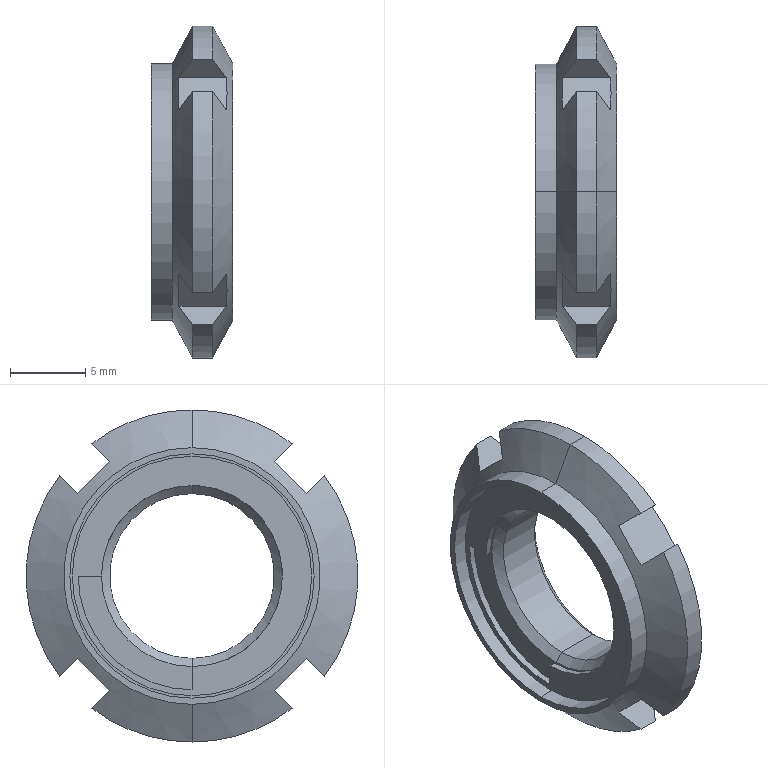Part | STEP file | Lock nut FUNT12_MISUMI | 2 solids | 42 faces | box 5.4 x 22 x 22 mm | volume 932.86 mm3 | plane 19 | cylinder 15 | cone 8 | commonest cylinder face diameters 22 x5 10.917 x2 15.867 x2 16.19 x2 17 x2 12 x1
STEP:
#1=CARTESIAN_POINT('',(-4.14,0.,-7.933));
#2=VERTEX_POINT('',#1);
#3=CARTESIAN_POINT('',(-4.14,0.,7.933));
#4=VERTEX_POINT('',#3);
#5=CARTESIAN_POINT('',(-4.14,0.,0.));
#6=DIRECTION('',(1.,0.,0.));
#7=DIRECTION('',(0.,0.,1.));
#8=AXIS2_PLACEMENT_3D('',#5,#6,#7);
#9=CIRCLE('',#8,7.933);
#10=EDGE_CURVE('',#2,#4,#9,.T.);
#11=ORIENTED_EDGE('',*,*,#10,.F.);
#12=CARTESIAN_POINT('',(-4.56,0.,-7.933));
#13=VERTEX_POINT('',#12);
#14=CARTESIAN_POINT('',(-4.14,0.,-7.933));
#15=DIRECTION('',(-1.,0.,0.));
#16=VECTOR('',#15,1000.);
#17=LINE('',#14,#16);
#18=EDGE_CURVE('',#2,#13,#17,.T.);
#19=ORIENTED_EDGE('',*,*,#18,.T.);
#20=CARTESIAN_POINT('',(-4.56,0.,7.933));
#21=VERTEX_POINT('',#20);
#22=CARTESIAN_POINT('',(-4.56,0.,0.));
#23=DIRECTION('',(1.,0.,0.));
#24=DIRECTION('',(0.,0.,1.));
#25=AXIS2_PLACEMENT_3D('',#22,#23,#24);
#26=CIRCLE('',#25,7.933);
#27=EDGE_CURVE('',#13,#21,#26,.T.);
#28=ORIENTED_EDGE('',*,*,#27,.T.);
#29=CARTESIAN_POINT('',(-4.14,0.,7.933));
#30=DIRECTION('',(-1.,0.,0.));
#31=VECTOR('',#30,1000.);
#32=LINE('',#29,#31);
#33=EDGE_CURVE('',#4,#21,#32,.T.);
#34=ORIENTED_EDGE('',*,*,#33,.F.);
#35=EDGE_LOOP('',(#11,#19,#28,#34));
#36=FACE_OUTER_BOUND('',#35,.T.);
#37=CARTESIAN_POINT('',(-4.14,0.,0.));
#38=DIRECTION('',(-1.,0.,0.));
#39=DIRECTION('',(0.,0.,1.));
#40=AXIS2_PLACEMENT_3D('',#37,#38,#39);
#41=CYLINDRICAL_SURFACE('',#40,7.933);
#42=ADVANCED_FACE('',(#36),#41,.T.);
#43=CARTESIAN_POINT('',(-4.14,0.,0.));
#44=DIRECTION('',(1.,0.,0.));
#45=DIRECTION('',(0.,0.,1.));
#46=AXIS2_PLACEMENT_3D('',#43,#44,#45);
#47=CIRCLE('',#46,7.933);
#48=EDGE_CURVE('',#4,#2,#47,.T.);
#49=ORIENTED_EDGE('',*,*,#48,.T.);
#50=ORIENTED_EDGE('',*,*,#10,.T.);
#51=EDGE_LOOP('',(#49,#50));
#52=FACE_OUTER_BOUND('',#51,.T.);
#53=CARTESIAN_POINT('',(-4.14,0.,-7.537));
#54=VERTEX_POINT('',#53);
#55=CARTESIAN_POINT('',(-4.14,0.,-6.));
#56=VERTEX_POINT('',#55);
#57=CARTESIAN_POINT('',(-4.14,0.,7.933));
#58=DIRECTION('',(0.,0.,1.));
#59=VECTOR('',#58,1000.);
#60=LINE('',#57,#59);
#61=EDGE_CURVE('',#54,#56,#60,.T.);
#62=ORIENTED_EDGE('',*,*,#61,.T.);
#63=CARTESIAN_POINT('',(-4.14,6.,0.));
#64=VERTEX_POINT('',#63);
#65=CARTESIAN_POINT('',(-4.14,0.,0.));
#66=DIRECTION('',(-1.,0.,0.));
#67=DIRECTION('',(0.,0.,-1.));
#68=AXIS2_PLACEMENT_3D('',#65,#66,#67);
#69=CIRCLE('',#68,6.);
#70=EDGE_CURVE('',#56,#64,#69,.T.);
#71=ORIENTED_EDGE('',*,*,#70,.T.);
#72=CARTESIAN_POINT('',(-4.14,7.537,0.));
#73=VERTEX_POINT('',#72);
#74=CARTESIAN_POINT('',(-4.14,-7.933,0.));
#75=DIRECTION('',(0.,1.,0.));
#76=VECTOR('',#75,1000.);
#77=LINE('',#74,#76);
#78=EDGE_CURVE('',#64,#73,#77,.T.);
#79=ORIENTED_EDGE('',*,*,#78,.T.);
#80=CARTESIAN_POINT('',(-4.14,0.,0.));
#81=DIRECTION('',(-1.,0.,0.));
#82=DIRECTION('',(0.,0.,-1.));
#83=AXIS2_PLACEMENT_3D('',#80,#81,#82);
#84=CIRCLE('',#83,7.537);
#85=EDGE_CURVE('',#73,#54,#84,.T.);
#86=ORIENTED_EDGE('',*,*,#85,.T.);
#87=EDGE_LOOP('',(#62,#71,#79,#86));
#88=FACE_BOUND('',#87,.T.);
#89=CARTESIAN_POINT('',(-4.14,-7.933,7.933));
#90=DIRECTION('',(1.,0.,0.));
#91=DIRECTION('',(0.,0.,-1.));
#92=AXIS2_PLACEMENT_3D('',#89,#90,#91);
#93=PLANE('',#92);
#94=ADVANCED_FACE('',(#52,#88),#93,.T.);
#95=ORIENTED_EDGE('',*,*,#18,.F.);
#96=ORIENTED_EDGE('',*,*,#48,.F.);
#97=ORIENTED_EDGE('',*,*,#33,.T.);
#98=CARTESIAN_POINT('',(-4.56,0.,0.));
#99=DIRECTION('',(1.,0.,0.));
#100=DIRECTION('',(0.,0.,1.));
#101=AXIS2_PLACEMENT_3D('',#98,#99,#100);
#102=CIRCLE('',#101,7.933);
#103=EDGE_CURVE('',#21,#13,#102,.T.);
#104=ORIENTED_EDGE('',*,*,#103,.T.);
#105=EDGE_LOOP('',(#95,#96,#97,#104));
#106=FACE_OUTER_BOUND('',#105,.T.);
#107=CARTESIAN_POINT('',(-4.14,0.,0.));
#108=DIRECTION('',(-1.,0.,0.));
#109=DIRECTION('',(0.,0.,1.));
#110=AXIS2_PLACEMENT_3D('',#107,#108,#109);
#111=CYLINDRICAL_SURFACE('',#110,7.933);
#112=ADVANCED_FACE('',(#106),#111,.T.);
#113=ORIENTED_EDGE('',*,*,#70,.F.);
#114=CARTESIAN_POINT('',(-4.56,0.,-6.));
#115=VERTEX_POINT('',#114);
#116=CARTESIAN_POINT('',(-4.56,0.,-6.));
#117=DIRECTION('',(1.,0.,0.));
#118=VECTOR('',#117,1000.);
#119=LINE('',#116,#118);
#120=EDGE_CURVE('',#115,#56,#119,.T.);
#121=ORIENTED_EDGE('',*,*,#120,.F.);
#122=CARTESIAN_POINT('',(-4.56,6.,0.));
#123=VERTEX_POINT('',#122);
#124=CARTESIAN_POINT('',(-4.56,0.,0.));
#125=DIRECTION('',(1.,0.,0.));
#126=DIRECTION('',(0.,0.,-1.));
#127=AXIS2_PLACEMENT_3D('',#124,#125,#126);
#128=CIRCLE('',#127,6.);
#129=EDGE_CURVE('',#123,#115,#128,.T.);
#130=ORIENTED_EDGE('',*,*,#129,.F.);
#131=CARTESIAN_POINT('',(-4.56,6.,0.));
#132=DIRECTION('',(-1.,0.,0.));
#133=VECTOR('',#132,1000.);
#134=LINE('',#131,#133);
#135=EDGE_CURVE('',#64,#123,#134,.T.);
#136=ORIENTED_EDGE('',*,*,#135,.F.);
#137=EDGE_LOOP('',(#113,#121,#130,#136));
#138=FACE_OUTER_BOUND('',#137,.T.);
#139=CARTESIAN_POINT('',(-4.56,0.,0.));
#140=DIRECTION('',(1.,0.,0.));
#141=DIRECTION('',(0.,0.,-1.));
#142=AXIS2_PLACEMENT_3D('',#139,#140,#141);
#143=CYLINDRICAL_SURFACE('',#142,6.);
#144=ADVANCED_FACE('',(#138),#143,.F.);
#145=ORIENTED_EDGE('',*,*,#120,.T.);
#146=ORIENTED_EDGE('',*,*,#61,.F.);
#147=CARTESIAN_POINT('',(-4.56,0.,-7.537));
#148=VERTEX_POINT('',#147);
#149=CARTESIAN_POINT('',(-4.14,0.,-7.537));
#150=DIRECTION('',(-1.,0.,0.));
#151=VECTOR('',#150,1000.);
#152=LINE('',#149,#151);
#153=EDGE_CURVE('',#54,#148,#152,.T.);
#154=ORIENTED_EDGE('',*,*,#153,.T.);
#155=CARTESIAN_POINT('',(-4.56,0.,-7.537));
#156=DIRECTION('',(0.,0.,1.));
#157=VECTOR('',#156,1000.);
#158=LINE('',#155,#157);
#159=EDGE_CURVE('',#148,#115,#158,.T.);
#160=ORIENTED_EDGE('',*,*,#159,.T.);
#161=EDGE_LOOP('',(#145,#146,#154,#160));
#162=FACE_OUTER_BOUND('',#161,.T.);
#163=CARTESIAN_POINT('',(-4.14,0.,-7.537));
#164=DIRECTION('',(0.,1.,0.));
#165=DIRECTION('',(0.,0.,1.));
#166=AXIS2_PLACEMENT_3D('',#163,#164,#165);
#167=PLANE('',#166);
#168=ADVANCED_FACE('',(#162),#167,.T.);
#169=CARTESIAN_POINT('',(-4.56,7.537,0.));
#170=VERTEX_POINT('',#169);
#171=CARTESIAN_POINT('',(-4.56,7.537,0.));
#172=DIRECTION('',(1.,0.,0.));
#173=VECTOR('',#172,1000.);
#174=LINE('',#171,#173);
#175=EDGE_CURVE('',#170,#73,#174,.T.);
#176=ORIENTED_EDGE('',*,*,#175,.F.);
#177=CARTESIAN_POINT('',(-4.56,0.,0.));
#178=DIRECTION('',(1.,0.,0.));
#179=DIRECTION('',(0.,0.,-1.));
#180=AXIS2_PLACEMENT_3D('',#177,#178,#179);
#181=CIRCLE('',#180,7.537);
#182=EDGE_CURVE('',#148,#170,#181,.T.);
#183=ORIENTED_EDGE('',*,*,#182,.F.);
#184=ORIENTED_EDGE('',*,*,#153,.F.);
#185=ORIENTED_EDGE('',*,*,#85,.F.);
#186=EDGE_LOOP('',(#176,#183,#184,#185));
#187=FACE_OUTER_BOUND('',#186,.T.);
#188=CARTESIAN_POINT('',(-4.56,0.,0.));
#189=DIRECTION('',(1.,0.,0.));
#190=DIRECTION('',(0.,0.,-1.));
#191=AXIS2_PLACEMENT_3D('',#188,#189,#190);
#192=CYLINDRICAL_SURFACE('',#191,7.537);
#193=ADVANCED_FACE('',(#187),#192,.F.);
#194=ORIENTED_EDGE('',*,*,#175,.T.);
#195=ORIENTED_EDGE('',*,*,#78,.F.);
#196=ORIENTED_EDGE('',*,*,#135,.T.);
#197=CARTESIAN_POINT('',(-4.56,6.,0.));
#198=DIRECTION('',(0.,1.,0.));
#199=VECTOR('',#198,1000.);
#200=LINE('',#197,#199);
#201=EDGE_CURVE('',#123,#170,#200,.T.);
#202=ORIENTED_EDGE('',*,*,#201,.T.);
#203=EDGE_LOOP('',(#194,#195,#196,#202));
#204=FACE_OUTER_BOUND('',#203,.T.);
#205=CARTESIAN_POINT('',(-4.14,6.,0.));
#206=DIRECTION('',(0.,0.,-1.));
#207=DIRECTION('',(0.,1.,0.));
#208=AXIS2_PLACEMENT_3D('',#205,#206,#207);
#209=PLANE('',#208);
#210=ADVANCED_FACE('',(#204),#209,.T.);
#211=ORIENTED_EDGE('',*,*,#103,.F.);
#212=ORIENTED_EDGE('',*,*,#27,.F.);
#213=EDGE_LOOP('',(#211,#212));
#214=FACE_OUTER_BOUND('',#213,.T.);
#215=ORIENTED_EDGE('',*,*,#159,.F.);
#216=ORIENTED_EDGE('',*,*,#182,.T.);
#217=ORIENTED_EDGE('',*,*,#201,.F.);
#218=ORIENTED_EDGE('',*,*,#129,.T.);
#219=EDGE_LOOP('',(#215,#216,#217,#218));
#220=FACE_BOUND('',#219,.T.);
#221=CARTESIAN_POINT('',(-4.56,-7.933,-7.933));
#222=DIRECTION('',(-1.,0.,0.));
#223=DIRECTION('',(0.,0.,1.));
#224=AXIS2_PLACEMENT_3D('',#221,#222,#223);
#225=PLANE('',#224);
#226=ADVANCED_FACE('',(#214,#220),#225,.T.);
#227=CLOSED_SHELL('',(#42,#94,#112,#144,#168,#193,#210,#226));
#228=MANIFOLD_SOLID_BREP('',#227);
#229=CARTESIAN_POINT('',(0.,0.,-8.5));
#230=VERTEX_POINT('',#229);
#231=CARTESIAN_POINT('',(0.,0.,8.5));
#232=VERTEX_POINT('',#231);
#233=CARTESIAN_POINT('',(0.,0.,0.));
#234=DIRECTION('',(1.,0.,0.));
#235=DIRECTION('',(0.,0.,1.));
#236=AXIS2_PLACEMENT_3D('',#233,#234,#235);
#237=CIRCLE('',#236,8.5);
#238=EDGE_CURVE('',#230,#232,#237,.T.);
#239=ORIENTED_EDGE('',*,*,#238,.F.);
#240=CARTESIAN_POINT('',(-1.333,0.,-11.));
#241=VERTEX_POINT('',#240);
#242=CARTESIAN_POINT('',(-1.333,0.,-11.));
#243=DIRECTION('',(-0.4706,0.,-0.8824));
#244=VECTOR('',#243,1000.);
#245=LINE('',#242,#244);
#246=EDGE_CURVE('',#230,#241,#245,.T.);
#247=ORIENTED_EDGE('',*,*,#246,.T.);
#248=CARTESIAN_POINT('',(-1.333,6.645,-8.766));
#249=VERTEX_POINT('',#248);
#250=CARTESIAN_POINT('',(-1.333,0.,0.));
#251=DIRECTION('',(1.,0.,0.));
#252=DIRECTION('',(0.,0.,1.));
#253=AXIS2_PLACEMENT_3D('',#250,#251,#252);
#254=CIRCLE('',#253,11.);
#255=EDGE_CURVE('',#241,#249,#254,.T.);
#256=ORIENTED_EDGE('',*,*,#255,.T.);
#257=CARTESIAN_POINT('',(-0.4381,5.445,-7.566));
#258=VERTEX_POINT('',#257);
#259=CARTESIAN_POINT('',(-1.333,6.645,-8.766));
#260=CARTESIAN_POINT('',(-1.035,6.245,-8.366));
#261=CARTESIAN_POINT('',(-0.7361,5.845,-7.966));
#262=CARTESIAN_POINT('',(-0.4381,5.445,-7.566));
#263=B_SPLINE_CURVE_WITH_KNOTS('',3,(#259,#260,#261,#262),.UNSPECIFIED.,.F.,.F.,(4,4),(0.,0.001919),.UNSPECIFIED.);
#264=EDGE_CURVE('',#249,#258,#263,.T.);
#265=ORIENTED_EDGE('',*,*,#264,.T.);
#266=CARTESIAN_POINT('',(-0.4381,7.566,-5.445));
#267=VERTEX_POINT('',#266);
#268=CARTESIAN_POINT('',(-0.4381,5.445,-7.566));
#269=CARTESIAN_POINT('',(-0.3523,6.152,-6.859));
#270=CARTESIAN_POINT('',(-0.3523,6.859,-6.152));
#271=CARTESIAN_POINT('',(-0.4381,7.566,-5.445));
#272=B_SPLINE_CURVE_WITH_KNOTS('',3,(#268,#269,#270,#271),.UNSPECIFIED.,.F.,.F.,(4,4),(0.,0.003),.UNSPECIFIED.);
#273=EDGE_CURVE('',#258,#267,#272,.T.);
#274=ORIENTED_EDGE('',*,*,#273,.T.);
#275=CARTESIAN_POINT('',(-1.333,8.766,-6.645));
#276=VERTEX_POINT('',#275);
#277=CARTESIAN_POINT('',(-0.4381,7.566,-5.445));
#278=CARTESIAN_POINT('',(-0.7361,7.966,-5.845));
#279=CARTESIAN_POINT('',(-1.035,8.366,-6.245));
#280=CARTESIAN_POINT('',(-1.333,8.766,-6.645));
#281=B_SPLINE_CURVE_WITH_KNOTS('',3,(#277,#278,#279,#280),.UNSPECIFIED.,.F.,.F.,(4,4),(0.,0.001919),.UNSPECIFIED.);
#282=EDGE_CURVE('',#267,#276,#281,.T.);
#283=ORIENTED_EDGE('',*,*,#282,.T.);
#284=CARTESIAN_POINT('',(-1.333,8.766,6.645));
#285=VERTEX_POINT('',#284);
#286=CARTESIAN_POINT('',(-1.333,0.,0.));
#287=DIRECTION('',(1.,0.,0.));
#288=DIRECTION('',(0.,0.,1.));
#289=AXIS2_PLACEMENT_3D('',#286,#287,#288);
#290=CIRCLE('',#289,11.);
#291=EDGE_CURVE('',#276,#285,#290,.T.);
#292=ORIENTED_EDGE('',*,*,#291,.T.);
#293=CARTESIAN_POINT('',(-0.4381,7.566,5.445));
#294=VERTEX_POINT('',#293);
#295=CARTESIAN_POINT('',(-1.333,8.766,6.645));
#296=CARTESIAN_POINT('',(-1.035,8.366,6.245));
#297=CARTESIAN_POINT('',(-0.7361,7.966,5.845));
#298=CARTESIAN_POINT('',(-0.4381,7.566,5.445));
#299=B_SPLINE_CURVE_WITH_KNOTS('',3,(#295,#296,#297,#298),.UNSPECIFIED.,.F.,.F.,(4,4),(0.,0.001919),.UNSPECIFIED.);
#300=EDGE_CURVE('',#285,#294,#299,.T.);
#301=ORIENTED_EDGE('',*,*,#300,.T.);
#302=CARTESIAN_POINT('',(-0.4381,5.445,7.566));
#303=VERTEX_POINT('',#302);
#304=CARTESIAN_POINT('',(-0.4381,7.566,5.445));
#305=CARTESIAN_POINT('',(-0.3523,6.859,6.152));
#306=CARTESIAN_POINT('',(-0.3523,6.152,6.859));
#307=CARTESIAN_POINT('',(-0.4381,5.445,7.566));
#308=B_SPLINE_CURVE_WITH_KNOTS('',3,(#304,#305,#306,#307),.UNSPECIFIED.,.F.,.F.,(4,4),(0.,0.003),.UNSPECIFIED.);
#309=EDGE_CURVE('',#294,#303,#308,.T.);
#310=ORIENTED_EDGE('',*,*,#309,.T.);
#311=CARTESIAN_POINT('',(-1.333,6.645,8.766));
#312=VERTEX_POINT('',#311);
#313=CARTESIAN_POINT('',(-0.4381,5.445,7.566));
#314=CARTESIAN_POINT('',(-0.7361,5.845,7.966));
#315=CARTESIAN_POINT('',(-1.035,6.245,8.366));
#316=CARTESIAN_POINT('',(-1.333,6.645,8.766));
#317=B_SPLINE_CURVE_WITH_KNOTS('',3,(#313,#314,#315,#316),.UNSPECIFIED.,.F.,.F.,(4,4),(0.,0.001919),.UNSPECIFIED.);
#318=EDGE_CURVE('',#303,#312,#317,.T.);
#319=ORIENTED_EDGE('',*,*,#318,.T.);
#320=CARTESIAN_POINT('',(-1.333,0.,11.));
#321=VERTEX_POINT('',#320);
#322=CARTESIAN_POINT('',(-1.333,0.,0.));
#323=DIRECTION('',(1.,0.,0.));
#324=DIRECTION('',(0.,0.,1.));
#325=AXIS2_PLACEMENT_3D('',#322,#323,#324);
#326=CIRCLE('',#325,11.);
#327=EDGE_CURVE('',#312,#321,#326,.T.);
#328=ORIENTED_EDGE('',*,*,#327,.T.);
#329=CARTESIAN_POINT('',(-1.333,0.,11.));
#330=DIRECTION('',(-0.4706,0.,0.8824));
#331=VECTOR('',#330,1000.);
#332=LINE('',#329,#331);
#333=EDGE_CURVE('',#232,#321,#332,.T.);
#334=ORIENTED_EDGE('',*,*,#333,.F.);
#335=EDGE_LOOP('',(#239,#247,#256,#265,#274,#283,#292,#301,#310,#319,#328,#334));
#336=FACE_OUTER_BOUND('',#335,.T.);
#337=CARTESIAN_POINT('',(-1.333,0.,0.));
#338=DIRECTION('',(-1.,0.,0.));
#339=DIRECTION('',(0.,0.,1.));
#340=AXIS2_PLACEMENT_3D('',#337,#338,#339);
#341=CONICAL_SURFACE('',#340,11.,1.081);
#342=ADVANCED_FACE('',(#336),#341,.T.);
#343=CARTESIAN_POINT('',(-0.5415,0.,5.459));
#344=VERTEX_POINT('',#343);
#345=CARTESIAN_POINT('',(-0.5415,0.,-5.459));
#346=VERTEX_POINT('',#345);
#347=CARTESIAN_POINT('',(-0.5415,0.,0.));
#348=DIRECTION('',(1.,0.,0.));
#349=DIRECTION('',(0.,0.,-1.));
#350=AXIS2_PLACEMENT_3D('',#347,#348,#349);
#351=CIRCLE('',#350,5.459);
#352=EDGE_CURVE('',#344,#346,#351,.T.);
#353=ORIENTED_EDGE('',*,*,#352,.F.);
#354=CARTESIAN_POINT('',(0.,0.,6.));
#355=VERTEX_POINT('',#354);
#356=CARTESIAN_POINT('',(0.,0.,6.));
#357=DIRECTION('',(0.7071,0.,0.7071));
#358=VECTOR('',#357,1000.);
#359=LINE('',#356,#358);
#360=EDGE_CURVE('',#344,#355,#359,.T.);
#361=ORIENTED_EDGE('',*,*,#360,.T.);
#362=CARTESIAN_POINT('',(0.,0.,-6.));
#363=VERTEX_POINT('',#362);
#364=CARTESIAN_POINT('',(0.,0.,0.));
#365=DIRECTION('',(-1.,0.,0.));
#366=DIRECTION('',(0.,0.,-1.));
#367=AXIS2_PLACEMENT_3D('',#364,#365,#366);
#368=CIRCLE('',#367,6.);
#369=EDGE_CURVE('',#363,#355,#368,.T.);
#370=ORIENTED_EDGE('',*,*,#369,.F.);
#371=CARTESIAN_POINT('',(0.,0.,-6.));
#372=DIRECTION('',(0.7071,0.,-0.7071));
#373=VECTOR('',#372,1000.);
#374=LINE('',#371,#373);
#375=EDGE_CURVE('',#346,#363,#374,.T.);
#376=ORIENTED_EDGE('',*,*,#375,.F.);
#377=EDGE_LOOP('',(#353,#361,#370,#376));
#378=FACE_OUTER_BOUND('',#377,.T.);
#379=CARTESIAN_POINT('',(0.,0.,0.));
#380=DIRECTION('',(1.,0.,0.));
#381=DIRECTION('',(0.,0.,-1.));
#382=AXIS2_PLACEMENT_3D('',#379,#380,#381);
#383=CONICAL_SURFACE('',#382,6.,0.7854);
#384=ADVANCED_FACE('',(#378),#383,.F.);
#385=CARTESIAN_POINT('',(-1.333,-6.645,8.766));
#386=VERTEX_POINT('',#385);
#387=CARTESIAN_POINT('',(-1.333,0.,0.));
#388=DIRECTION('',(1.,0.,0.));
#389=DIRECTION('',(0.,0.,1.));
#390=AXIS2_PLACEMENT_3D('',#387,#388,#389);
#391=CIRCLE('',#390,11.);
#392=EDGE_CURVE('',#321,#386,#391,.T.);
#393=ORIENTED_EDGE('',*,*,#392,.F.);
#394=CARTESIAN_POINT('',(-2.667,0.,11.));
#395=VERTEX_POINT('',#394);
#396=CARTESIAN_POINT('',(-1.333,0.,11.));
#397=DIRECTION('',(-1.,0.,0.));
#398=VECTOR('',#397,1000.);
#399=LINE('',#396,#398);
#400=EDGE_CURVE('',#321,#395,#399,.T.);
#401=ORIENTED_EDGE('',*,*,#400,.T.);
#402=CARTESIAN_POINT('',(-2.667,-6.645,8.766));
#403=VERTEX_POINT('',#402);
#404=CARTESIAN_POINT('',(-2.667,0.,0.));
#405=DIRECTION('',(1.,0.,0.));
#406=DIRECTION('',(0.,0.,1.));
#407=AXIS2_PLACEMENT_3D('',#404,#405,#406);
#408=CIRCLE('',#407,11.);
#409=EDGE_CURVE('',#395,#403,#408,.T.);
#410=ORIENTED_EDGE('',*,*,#409,.T.);
#411=CARTESIAN_POINT('',(-3.562,-6.645,8.766));
#412=DIRECTION('',(-1.,0.,0.));
#413=VECTOR('',#412,1000.);
#414=LINE('',#411,#413);
#415=EDGE_CURVE('',#386,#403,#414,.T.);
#416=ORIENTED_EDGE('',*,*,#415,.F.);
#417=EDGE_LOOP('',(#393,#401,#410,#416));
#418=FACE_OUTER_BOUND('',#417,.T.);
#419=CARTESIAN_POINT('',(-1.333,0.,0.));
#420=DIRECTION('',(-1.,0.,0.));
#421=DIRECTION('',(0.,0.,1.));
#422=AXIS2_PLACEMENT_3D('',#419,#420,#421);
#423=CYLINDRICAL_SURFACE('',#422,11.);
#424=ADVANCED_FACE('',(#418),#423,.T.);
#425=ORIENTED_EDGE('',*,*,#352,.T.);
#426=CARTESIAN_POINT('',(-3.459,0.,-5.459));
#427=VERTEX_POINT('',#426);
#428=CARTESIAN_POINT('',(-0.5415,0.,-5.459));
#429=DIRECTION('',(-1.,0.,0.));
#430=VECTOR('',#429,1000.);
#431=LINE('',#428,#430);
#432=EDGE_CURVE('',#346,#427,#431,.T.);
#433=ORIENTED_EDGE('',*,*,#432,.T.);
#434=CARTESIAN_POINT('',(-3.459,0.,5.458));
#435=VERTEX_POINT('',#434);
#436=CARTESIAN_POINT('',(-3.459,0.,0.));
#437=DIRECTION('',(1.,0.,0.));
#438=DIRECTION('',(0.,0.,1.));
#439=AXIS2_PLACEMENT_3D('',#436,#437,#438);
#440=CIRCLE('',#439,5.458);
#441=EDGE_CURVE('',#435,#427,#440,.T.);
#442=ORIENTED_EDGE('',*,*,#441,.F.);
#443=CARTESIAN_POINT('',(-0.5415,0.,5.458));
#444=DIRECTION('',(-1.,0.,0.));
#445=VECTOR('',#444,1000.);
#446=LINE('',#443,#445);
#447=EDGE_CURVE('',#344,#435,#446,.T.);
#448=ORIENTED_EDGE('',*,*,#447,.F.);
#449=EDGE_LOOP('',(#425,#433,#442,#448));
#450=FACE_OUTER_BOUND('',#449,.T.);
#451=CARTESIAN_POINT('',(-0.5415,0.,0.));
#452=DIRECTION('',(-1.,0.,0.));
#453=DIRECTION('',(0.,0.,1.));
#454=AXIS2_PLACEMENT_3D('',#451,#452,#453);
#455=CYLINDRICAL_SURFACE('',#454,5.458);
#456=ADVANCED_FACE('',(#450),#455,.F.);
#457=CARTESIAN_POINT('',(-4.,0.,-8.5));
#458=VERTEX_POINT('',#457);
#459=CARTESIAN_POINT('',(-4.,0.,8.5));
#460=VERTEX_POINT('',#459);
#461=CARTESIAN_POINT('',(-4.,0.,0.));
#462=DIRECTION('',(1.,0.,0.));
#463=DIRECTION('',(0.,0.,-1.));
#464=AXIS2_PLACEMENT_3D('',#461,#462,#463);
#465=CIRCLE('',#464,8.5);
#466=EDGE_CURVE('',#458,#460,#465,.T.);
#467=ORIENTED_EDGE('',*,*,#466,.T.);
#468=CARTESIAN_POINT('',(-2.667,0.,11.));
#469=DIRECTION('',(0.4706,0.,0.8824));
#470=VECTOR('',#469,1000.);
#471=LINE('',#468,#470);
#472=EDGE_CURVE('',#460,#395,#471,.T.);
#473=ORIENTED_EDGE('',*,*,#472,.T.);
#474=CARTESIAN_POINT('',(-2.667,6.645,8.766));
#475=VERTEX_POINT('',#474);
#476=CARTESIAN_POINT('',(-2.667,0.,0.));
#477=DIRECTION('',(1.,0.,0.));
#478=DIRECTION('',(0.,0.,1.));
#479=AXIS2_PLACEMENT_3D('',#476,#477,#478);
#480=CIRCLE('',#479,11.);
#481=EDGE_CURVE('',#475,#395,#480,.T.);
#482=ORIENTED_EDGE('',*,*,#481,.F.);
#483=CARTESIAN_POINT('',(-3.562,5.445,7.566));
#484=VERTEX_POINT('',#483);
#485=CARTESIAN_POINT('',(-3.562,5.445,7.566));
#486=CARTESIAN_POINT('',(-3.264,5.845,7.966));
#487=CARTESIAN_POINT('',(-2.965,6.245,8.366));
#488=CARTESIAN_POINT('',(-2.667,6.645,8.766));
#489=B_SPLINE_CURVE_WITH_KNOTS('',3,(#485,#486,#487,#488),.UNSPECIFIED.,.F.,.F.,(4,4),(0.,0.001919),.UNSPECIFIED.);
#490=EDGE_CURVE('',#484,#475,#489,.T.);
#491=ORIENTED_EDGE('',*,*,#490,.F.);
#492=CARTESIAN_POINT('',(-3.562,7.566,5.445));
#493=VERTEX_POINT('',#492);
#494=CARTESIAN_POINT('',(-3.562,7.566,5.445));
#495=CARTESIAN_POINT('',(-3.648,6.859,6.152));
#496=CARTESIAN_POINT('',(-3.648,6.152,6.859));
#497=CARTESIAN_POINT('',(-3.562,5.445,7.566));
#498=B_SPLINE_CURVE_WITH_KNOTS('',3,(#494,#495,#496,#497),.UNSPECIFIED.,.F.,.F.,(4,4),(0.,0.003),.UNSPECIFIED.);
#499=EDGE_CURVE('',#493,#484,#498,.T.);
#500=ORIENTED_EDGE('',*,*,#499,.F.);
#501=CARTESIAN_POINT('',(-2.667,8.766,6.645));
#502=VERTEX_POINT('',#501);
#503=CARTESIAN_POINT('',(-2.667,8.766,6.645));
#504=CARTESIAN_POINT('',(-2.965,8.366,6.245));
#505=CARTESIAN_POINT('',(-3.264,7.966,5.845));
#506=CARTESIAN_POINT('',(-3.562,7.566,5.445));
#507=B_SPLINE_CURVE_WITH_KNOTS('',3,(#503,#504,#505,#506),.UNSPECIFIED.,.F.,.F.,(4,4),(0.,0.001919),.UNSPECIFIED.);
#508=EDGE_CURVE('',#502,#493,#507,.T.);
#509=ORIENTED_EDGE('',*,*,#508,.F.);
#510=CARTESIAN_POINT('',(-2.667,8.766,-6.645));
#511=VERTEX_POINT('',#510);
#512=CARTESIAN_POINT('',(-2.667,0.,0.));
#513=DIRECTION('',(1.,0.,0.));
#514=DIRECTION('',(0.,0.,1.));
#515=AXIS2_PLACEMENT_3D('',#512,#513,#514);
#516=CIRCLE('',#515,11.);
#517=EDGE_CURVE('',#511,#502,#516,.T.);
#518=ORIENTED_EDGE('',*,*,#517,.F.);
#519=CARTESIAN_POINT('',(-3.562,7.566,-5.445));
#520=VERTEX_POINT('',#519);
#521=CARTESIAN_POINT('',(-3.562,7.566,-5.445));
#522=CARTESIAN_POINT('',(-3.264,7.966,-5.845));
#523=CARTESIAN_POINT('',(-2.965,8.366,-6.245));
#524=CARTESIAN_POINT('',(-2.667,8.766,-6.645));
#525=B_SPLINE_CURVE_WITH_KNOTS('',3,(#521,#522,#523,#524),.UNSPECIFIED.,.F.,.F.,(4,4),(0.,0.001919),.UNSPECIFIED.);
#526=EDGE_CURVE('',#520,#511,#525,.T.);
#527=ORIENTED_EDGE('',*,*,#526,.F.);
#528=CARTESIAN_POINT('',(-3.562,5.445,-7.566));
#529=VERTEX_POINT('',#528);
#530=CARTESIAN_POINT('',(-3.562,5.445,-7.566));
#531=CARTESIAN_POINT('',(-3.648,6.152,-6.859));
#532=CARTESIAN_POINT('',(-3.648,6.859,-6.152));
#533=CARTESIAN_POINT('',(-3.562,7.566,-5.445));
#534=B_SPLINE_CURVE_WITH_KNOTS('',3,(#530,#531,#532,#533),.UNSPECIFIED.,.F.,.F.,(4,4),(0.,0.003),.UNSPECIFIED.);
#535=EDGE_CURVE('',#529,#520,#534,.T.);
#536=ORIENTED_EDGE('',*,*,#535,.F.);
#537=CARTESIAN_POINT('',(-2.667,6.645,-8.766));
#538=VERTEX_POINT('',#537);
#539=CARTESIAN_POINT('',(-2.667,6.645,-8.766));
#540=CARTESIAN_POINT('',(-2.965,6.245,-8.366));
#541=CARTESIAN_POINT('',(-3.264,5.845,-7.966));
#542=CARTESIAN_POINT('',(-3.562,5.445,-7.566));
#543=B_SPLINE_CURVE_WITH_KNOTS('',3,(#539,#540,#541,#542),.UNSPECIFIED.,.F.,.F.,(4,4),(0.,0.001919),.UNSPECIFIED.);
#544=EDGE_CURVE('',#538,#529,#543,.T.);
#545=ORIENTED_EDGE('',*,*,#544,.F.);
#546=CARTESIAN_POINT('',(-2.667,0.,-11.));
#547=VERTEX_POINT('',#546);
#548=CARTESIAN_POINT('',(-2.667,0.,0.));
#549=DIRECTION('',(1.,0.,0.));
#550=DIRECTION('',(0.,0.,1.));
#551=AXIS2_PLACEMENT_3D('',#548,#549,#550);
#552=CIRCLE('',#551,11.);
#553=EDGE_CURVE('',#547,#538,#552,.T.);
#554=ORIENTED_EDGE('',*,*,#553,.F.);
#555=CARTESIAN_POINT('',(-2.667,0.,-11.));
#556=DIRECTION('',(0.4706,0.,-0.8824));
#557=VECTOR('',#556,1000.);
#558=LINE('',#555,#557);
#559=EDGE_CURVE('',#458,#547,#558,.T.);
#560=ORIENTED_EDGE('',*,*,#559,.F.);
#561=EDGE_LOOP('',(#467,#473,#482,#491,#500,#509,#518,#527,#536,#545,#554,#560));
#562=FACE_OUTER_BOUND('',#561,.T.);
#563=CARTESIAN_POINT('',(-2.667,0.,0.));
#564=DIRECTION('',(1.,0.,0.));
#565=DIRECTION('',(0.,0.,-1.));
#566=AXIS2_PLACEMENT_3D('',#563,#564,#565);
#567=CONICAL_SURFACE('',#566,11.,1.081);
#568=ADVANCED_FACE('',(#562),#567,.T.);
#569=ORIENTED_EDGE('',*,*,#441,.T.);
#570=CARTESIAN_POINT('',(-4.,0.,-6.));
#571=VERTEX_POINT('',#570);
#572=CARTESIAN_POINT('',(-4.,0.,-6.));
#573=DIRECTION('',(-0.7071,0.,-0.7071));
#574=VECTOR('',#573,1000.);
#575=LINE('',#572,#574);
#576=EDGE_CURVE('',#427,#571,#575,.T.);
#577=ORIENTED_EDGE('',*,*,#576,.T.);
#578=CARTESIAN_POINT('',(-4.,0.,6.));
#579=VERTEX_POINT('',#578);
#580=CARTESIAN_POINT('',(-4.,0.,0.));
#581=DIRECTION('',(1.,0.,0.));
#582=DIRECTION('',(0.,0.,1.));
#583=AXIS2_PLACEMENT_3D('',#580,#581,#582);
#584=CIRCLE('',#583,6.);
#585=EDGE_CURVE('',#579,#571,#584,.T.);
#586=ORIENTED_EDGE('',*,*,#585,.F.);
#587=CARTESIAN_POINT('',(-4.,0.,6.));
#588=DIRECTION('',(-0.7071,0.,0.7071));
#589=VECTOR('',#588,1000.);
#590=LINE('',#587,#589);
#591=EDGE_CURVE('',#435,#579,#590,.T.);
#592=ORIENTED_EDGE('',*,*,#591,.F.);
#593=EDGE_LOOP('',(#569,#577,#586,#592));
#594=FACE_OUTER_BOUND('',#593,.T.);
#595=CARTESIAN_POINT('',(-4.,0.,0.));
#596=DIRECTION('',(-1.,0.,0.));
#597=DIRECTION('',(0.,0.,1.));
#598=AXIS2_PLACEMENT_3D('',#595,#596,#597);
#599=CONICAL_SURFACE('',#598,6.,0.7854);
#600=ADVANCED_FACE('',(#594),#599,.F.);
#601=ORIENTED_EDGE('',*,*,#466,.F.);
#602=CARTESIAN_POINT('',(-5.4,0.,-8.5));
#603=VERTEX_POINT('',#602);
#604=CARTESIAN_POINT('',(-4.,0.,-8.5));
#605=DIRECTION('',(-1.,0.,0.));
#606=VECTOR('',#605,1000.);
#607=LINE('',#604,#606);
#608=EDGE_CURVE('',#458,#603,#607,.T.);
#609=ORIENTED_EDGE('',*,*,#608,.T.);
#610=CARTESIAN_POINT('',(-5.4,0.,8.5));
#611=VERTEX_POINT('',#610);
#612=CARTESIAN_POINT('',(-5.4,0.,0.));
#613=DIRECTION('',(1.,0.,0.));
#614=DIRECTION('',(0.,0.,1.));
#615=AXIS2_PLACEMENT_3D('',#612,#613,#614);
#616=CIRCLE('',#615,8.5);
#617=EDGE_CURVE('',#603,#611,#616,.T.);
#618=ORIENTED_EDGE('',*,*,#617,.T.);
#619=CARTESIAN_POINT('',(-4.,0.,8.5));
#620=DIRECTION('',(-1.,0.,0.));
#621=VECTOR('',#620,1000.);
#622=LINE('',#619,#621);
#623=EDGE_CURVE('',#460,#611,#622,.T.);
#624=ORIENTED_EDGE('',*,*,#623,.F.);
#625=EDGE_LOOP('',(#601,#609,#618,#624));
#626=FACE_OUTER_BOUND('',#625,.T.);
#627=CARTESIAN_POINT('',(-4.,0.,0.));
#628=DIRECTION('',(-1.,0.,0.));
#629=DIRECTION('',(0.,0.,1.));
#630=AXIS2_PLACEMENT_3D('',#627,#628,#629);
#631=CYLINDRICAL_SURFACE('',#630,8.5);
#632=ADVANCED_FACE('',(#626),#631,.T.);
#633=CARTESIAN_POINT('',(-5.4,0.,8.095));
#634=VERTEX_POINT('',#633);
#635=CARTESIAN_POINT('',(-5.4,0.,-8.095));
#636=VERTEX_POINT('',#635);
#637=CARTESIAN_POINT('',(-5.4,0.,0.));
#638=DIRECTION('',(1.,0.,0.));
#639=DIRECTION('',(0.,0.,-1.));
#640=AXIS2_PLACEMENT_3D('',#637,#638,#639);
#641=CIRCLE('',#640,8.095);
#642=EDGE_CURVE('',#634,#636,#641,.T.);
#643=ORIENTED_EDGE('',*,*,#642,.F.);
#644=CARTESIAN_POINT('',(-4.,0.,8.095));
#645=VERTEX_POINT('',#644);
#646=CARTESIAN_POINT('',(-5.4,0.,8.095));
#647=DIRECTION('',(1.,0.,0.));
#648=VECTOR('',#647,1000.);
#649=LINE('',#646,#648);
#650=EDGE_CURVE('',#634,#645,#649,.T.);
#651=ORIENTED_EDGE('',*,*,#650,.T.);
#652=CARTESIAN_POINT('',(-4.,0.,-8.095));
#653=VERTEX_POINT('',#652);
#654=CARTESIAN_POINT('',(-4.,0.,0.));
#655=DIRECTION('',(-1.,0.,0.));
#656=DIRECTION('',(0.,0.,-1.));
#657=AXIS2_PLACEMENT_3D('',#654,#655,#656);
#658=CIRCLE('',#657,8.095);
#659=EDGE_CURVE('',#653,#645,#658,.T.);
#660=ORIENTED_EDGE('',*,*,#659,.F.);
#661=CARTESIAN_POINT('',(-5.4,0.,-8.095));
#662=DIRECTION('',(1.,0.,0.));
#663=VECTOR('',#662,1000.);
#664=LINE('',#661,#663);
#665=EDGE_CURVE('',#636,#653,#664,.T.);
#666=ORIENTED_EDGE('',*,*,#665,.F.);
#667=EDGE_LOOP('',(#643,#651,#660,#666));
#668=FACE_OUTER_BOUND('',#667,.T.);
#669=CARTESIAN_POINT('',(-5.4,0.,0.));
#670=DIRECTION('',(1.,0.,0.));
#671=DIRECTION('',(0.,0.,-1.));
#672=AXIS2_PLACEMENT_3D('',#669,#670,#671);
#673=CYLINDRICAL_SURFACE('',#672,8.095);
#674=ADVANCED_FACE('',(#668),#673,.F.);
#675=CARTESIAN_POINT('',(0.,0.,0.));
#676=DIRECTION('',(1.,0.,0.));
#677=DIRECTION('',(0.,0.,1.));
#678=AXIS2_PLACEMENT_3D('',#675,#676,#677);
#679=CIRCLE('',#678,8.5);
#680=EDGE_CURVE('',#232,#230,#679,.T.);
#681=ORIENTED_EDGE('',*,*,#680,.T.);
#682=ORIENTED_EDGE('',*,*,#238,.T.);
#683=EDGE_LOOP('',(#681,#682));
#684=FACE_OUTER_BOUND('',#683,.T.);
#685=ORIENTED_EDGE('',*,*,#369,.T.);
#686=CARTESIAN_POINT('',(0.,0.,0.));
#687=DIRECTION('',(-1.,0.,0.));
#688=DIRECTION('',(0.,0.,-1.));
#689=AXIS2_PLACEMENT_3D('',#686,#687,#688);
#690=CIRCLE('',#689,6.);
#691=EDGE_CURVE('',#355,#363,#690,.T.);
#692=ORIENTED_EDGE('',*,*,#691,.T.);
#693=EDGE_LOOP('',(#685,#692));
#694=FACE_BOUND('',#693,.T.);
#695=CARTESIAN_POINT('',(0.,-8.5,8.5));
#696=DIRECTION('',(1.,0.,0.));
#697=DIRECTION('',(0.,0.,-1.));
#698=AXIS2_PLACEMENT_3D('',#695,#696,#697);
#699=PLANE('',#698);
#700=ADVANCED_FACE('',(#684,#694),#699,.T.);
#701=ORIENTED_EDGE('',*,*,#246,.F.);
#702=ORIENTED_EDGE('',*,*,#680,.F.);
#703=ORIENTED_EDGE('',*,*,#333,.T.);
#704=ORIENTED_EDGE('',*,*,#392,.T.);
#705=CARTESIAN_POINT('',(-0.4381,-5.445,7.566));
#706=VERTEX_POINT('',#705);
#707=CARTESIAN_POINT('',(-1.333,-6.645,8.766));
#708=CARTESIAN_POINT('',(-1.035,-6.245,8.366));
#709=CARTESIAN_POINT('',(-0.7361,-5.845,7.966));
#710=CARTESIAN_POINT('',(-0.4381,-5.445,7.566));
#711=B_SPLINE_CURVE_WITH_KNOTS('',3,(#707,#708,#709,#710),.UNSPECIFIED.,.F.,.F.,(4,4),(0.,0.001919),.UNSPECIFIED.);
#712=EDGE_CURVE('',#386,#706,#711,.T.);
#713=ORIENTED_EDGE('',*,*,#712,.T.);
#714=CARTESIAN_POINT('',(-0.4381,-7.566,5.445));
#715=VERTEX_POINT('',#714);
#716=CARTESIAN_POINT('',(-0.4381,-5.445,7.566));
#717=CARTESIAN_POINT('',(-0.3523,-6.152,6.859));
#718=CARTESIAN_POINT('',(-0.3523,-6.859,6.152));
#719=CARTESIAN_POINT('',(-0.4381,-7.566,5.445));
#720=B_SPLINE_CURVE_WITH_KNOTS('',3,(#716,#717,#718,#719),.UNSPECIFIED.,.F.,.F.,(4,4),(0.,0.003),.UNSPECIFIED.);
#721=EDGE_CURVE('',#706,#715,#720,.T.);
#722=ORIENTED_EDGE('',*,*,#721,.T.);
#723=CARTESIAN_POINT('',(-1.333,-8.766,6.645));
#724=VERTEX_POINT('',#723);
#725=CARTESIAN_POINT('',(-0.4381,-7.566,5.445));
#726=CARTESIAN_POINT('',(-0.7361,-7.966,5.845));
#727=CARTESIAN_POINT('',(-1.035,-8.366,6.245));
#728=CARTESIAN_POINT('',(-1.333,-8.766,6.645));
#729=B_SPLINE_CURVE_WITH_KNOTS('',3,(#725,#726,#727,#728),.UNSPECIFIED.,.F.,.F.,(4,4),(0.,0.001919),.UNSPECIFIED.);
#730=EDGE_CURVE('',#715,#724,#729,.T.);
#731=ORIENTED_EDGE('',*,*,#730,.T.);
#732=CARTESIAN_POINT('',(-1.333,-8.766,-6.645));
#733=VERTEX_POINT('',#732);
#734=CARTESIAN_POINT('',(-1.333,0.,0.));
#735=DIRECTION('',(1.,0.,0.));
#736=DIRECTION('',(0.,0.,1.));
#737=AXIS2_PLACEMENT_3D('',#734,#735,#736);
#738=CIRCLE('',#737,11.);
#739=EDGE_CURVE('',#724,#733,#738,.T.);
#740=ORIENTED_EDGE('',*,*,#739,.T.);
#741=CARTESIAN_POINT('',(-0.4381,-7.566,-5.445));
#742=VERTEX_POINT('',#741);
#743=CARTESIAN_POINT('',(-1.333,-8.766,-6.645));
#744=CARTESIAN_POINT('',(-1.035,-8.366,-6.245));
#745=CARTESIAN_POINT('',(-0.7361,-7.966,-5.845));
#746=CARTESIAN_POINT('',(-0.4381,-7.566,-5.445));
#747=B_SPLINE_CURVE_WITH_KNOTS('',3,(#743,#744,#745,#746),.UNSPECIFIED.,.F.,.F.,(4,4),(0.,0.001919),.UNSPECIFIED.);
#748=EDGE_CURVE('',#733,#742,#747,.T.);
#749=ORIENTED_EDGE('',*,*,#748,.T.);
#750=CARTESIAN_POINT('',(-0.4381,-5.445,-7.566));
#751=VERTEX_POINT('',#750);
#752=CARTESIAN_POINT('',(-0.4381,-7.566,-5.445));
#753=CARTESIAN_POINT('',(-0.3523,-6.859,-6.152));
#754=CARTESIAN_POINT('',(-0.3523,-6.152,-6.859));
#755=CARTESIAN_POINT('',(-0.4381,-5.445,-7.566));
#756=B_SPLINE_CURVE_WITH_KNOTS('',3,(#752,#753,#754,#755),.UNSPECIFIED.,.F.,.F.,(4,4),(0.,0.003),.UNSPECIFIED.);
#757=EDGE_CURVE('',#742,#751,#756,.T.);
#758=ORIENTED_EDGE('',*,*,#757,.T.);
#759=CARTESIAN_POINT('',(-1.333,-6.645,-8.766));
#760=VERTEX_POINT('',#759);
#761=CARTESIAN_POINT('',(-0.4381,-5.445,-7.566));
#762=CARTESIAN_POINT('',(-0.7361,-5.845,-7.966));
#763=CARTESIAN_POINT('',(-1.035,-6.245,-8.366));
#764=CARTESIAN_POINT('',(-1.333,-6.645,-8.766));
#765=B_SPLINE_CURVE_WITH_KNOTS('',3,(#761,#762,#763,#764),.UNSPECIFIED.,.F.,.F.,(4,4),(0.,0.001919),.UNSPECIFIED.);
#766=EDGE_CURVE('',#751,#760,#765,.T.);
#767=ORIENTED_EDGE('',*,*,#766,.T.);
#768=CARTESIAN_POINT('',(-1.333,0.,0.));
#769=DIRECTION('',(1.,0.,0.));
#770=DIRECTION('',(0.,0.,1.));
#771=AXIS2_PLACEMENT_3D('',#768,#769,#770);
#772=CIRCLE('',#771,11.);
#773=EDGE_CURVE('',#760,#241,#772,.T.);
#774=ORIENTED_EDGE('',*,*,#773,.T.);
#775=EDGE_LOOP('',(#701,#702,#703,#704,#713,#722,#731,#740,#749,#758,#767,#774));
#776=FACE_OUTER_BOUND('',#775,.T.);
#777=CARTESIAN_POINT('',(-1.333,0.,0.));
#778=DIRECTION('',(-1.,0.,0.));
#779=DIRECTION('',(0.,0.,1.));
#780=AXIS2_PLACEMENT_3D('',#777,#778,#779);
#781=CONICAL_SURFACE('',#780,11.,1.081);
#782=ADVANCED_FACE('',(#776),#781,.T.);
#783=ORIENTED_EDGE('',*,*,#360,.F.);
#784=CARTESIAN_POINT('',(-0.5415,0.,0.));
#785=DIRECTION('',(1.,0.,0.));
#786=DIRECTION('',(0.,0.,-1.));
#787=AXIS2_PLACEMENT_3D('',#784,#785,#786);
#788=CIRCLE('',#787,5.459);
#789=EDGE_CURVE('',#346,#344,#788,.T.);
#790=ORIENTED_EDGE('',*,*,#789,.F.);
#791=ORIENTED_EDGE('',*,*,#375,.T.);
#792=ORIENTED_EDGE('',*,*,#691,.F.);
#793=EDGE_LOOP('',(#783,#790,#791,#792));
#794=FACE_OUTER_BOUND('',#793,.T.);
#795=CARTESIAN_POINT('',(0.,0.,0.));
#796=DIRECTION('',(1.,0.,0.));
#797=DIRECTION('',(0.,0.,-1.));
#798=AXIS2_PLACEMENT_3D('',#795,#796,#797);
#799=CONICAL_SURFACE('',#798,6.,0.7854);
#800=ADVANCED_FACE('',(#794),#799,.F.);
#801=CARTESIAN_POINT('',(-1.333,6.645,-8.766));
#802=DIRECTION('',(1.,0.,0.));
#803=VECTOR('',#802,1000.);
#804=LINE('',#801,#803);
#805=EDGE_CURVE('',#538,#249,#804,.T.);
#806=ORIENTED_EDGE('',*,*,#805,.T.);
#807=ORIENTED_EDGE('',*,*,#255,.F.);
#808=ORIENTED_EDGE('',*,*,#773,.F.);
#809=CARTESIAN_POINT('',(-2.667,-6.645,-8.766));
#810=VERTEX_POINT('',#809);
#811=CARTESIAN_POINT('',(-1.333,-6.645,-8.766));
#812=DIRECTION('',(-1.,0.,0.));
#813=VECTOR('',#812,1000.);
#814=LINE('',#811,#813);
#815=EDGE_CURVE('',#760,#810,#814,.T.);
#816=ORIENTED_EDGE('',*,*,#815,.T.);
#817=CARTESIAN_POINT('',(-2.667,0.,0.));
#818=DIRECTION('',(1.,0.,0.));
#819=DIRECTION('',(0.,0.,1.));
#820=AXIS2_PLACEMENT_3D('',#817,#818,#819);
#821=CIRCLE('',#820,11.);
#822=EDGE_CURVE('',#810,#547,#821,.T.);
#823=ORIENTED_EDGE('',*,*,#822,.T.);
#824=ORIENTED_EDGE('',*,*,#553,.T.);
#825=EDGE_LOOP('',(#806,#807,#808,#816,#823,#824));
#826=FACE_OUTER_BOUND('',#825,.T.);
#827=CARTESIAN_POINT('',(-1.333,0.,0.));
#828=DIRECTION('',(-1.,0.,0.));
#829=DIRECTION('',(0.,0.,1.));
#830=AXIS2_PLACEMENT_3D('',#827,#828,#829);
#831=CYLINDRICAL_SURFACE('',#830,11.);
#832=ADVANCED_FACE('',(#826),#831,.T.);
#833=CARTESIAN_POINT('',(-3.562,-5.445,-7.566));
#834=VERTEX_POINT('',#833);
#835=CARTESIAN_POINT('',(-3.562,-5.445,-7.566));
#836=CARTESIAN_POINT('',(-3.264,-5.845,-7.966));
#837=CARTESIAN_POINT('',(-2.965,-6.245,-8.366));
#838=CARTESIAN_POINT('',(-2.667,-6.645,-8.766));
#839=B_SPLINE_CURVE_WITH_KNOTS('',3,(#835,#836,#837,#838),.UNSPECIFIED.,.F.,.F.,(4,4),(0.,0.001919),.UNSPECIFIED.);
#840=EDGE_CURVE('',#834,#810,#839,.T.);
#841=ORIENTED_EDGE('',*,*,#840,.T.);
#842=ORIENTED_EDGE('',*,*,#815,.F.);
#843=ORIENTED_EDGE('',*,*,#766,.F.);
#844=CARTESIAN_POINT('',(-3.562,-5.445,-7.566));
#845=DIRECTION('',(-1.,0.,0.));
#846=VECTOR('',#845,1000.);
#847=LINE('',#844,#846);
#848=EDGE_CURVE('',#751,#834,#847,.T.);
#849=ORIENTED_EDGE('',*,*,#848,.T.);
#850=EDGE_LOOP('',(#841,#842,#843,#849));
#851=FACE_OUTER_BOUND('',#850,.T.);
#852=CARTESIAN_POINT('',(-3.562,-5.445,-7.566));
#853=DIRECTION('',(0.,-0.7071,0.7071));
#854=DIRECTION('',(0.,-0.7071,-0.7071));
#855=AXIS2_PLACEMENT_3D('',#852,#853,#854);
#856=PLANE('',#855);
#857=ADVANCED_FACE('',(#851),#856,.T.);
#858=CARTESIAN_POINT('',(-3.562,-7.566,-5.445));
#859=VERTEX_POINT('',#858);
#860=CARTESIAN_POINT('',(-3.562,-7.566,-5.445));
#861=CARTESIAN_POINT('',(-3.648,-6.859,-6.152));
#862=CARTESIAN_POINT('',(-3.648,-6.152,-6.859));
#863=CARTESIAN_POINT('',(-3.562,-5.445,-7.566));
#864=B_SPLINE_CURVE_WITH_KNOTS('',3,(#860,#861,#862,#863),.UNSPECIFIED.,.F.,.F.,(4,4),(0.,0.003),.UNSPECIFIED.);
#865=EDGE_CURVE('',#859,#834,#864,.T.);
#866=ORIENTED_EDGE('',*,*,#865,.T.);
#867=ORIENTED_EDGE('',*,*,#848,.F.);
#868=ORIENTED_EDGE('',*,*,#757,.F.);
#869=CARTESIAN_POINT('',(-3.691,-7.566,-5.445));
#870=DIRECTION('',(-1.,0.,0.));
#871=VECTOR('',#870,1000.);
#872=LINE('',#869,#871);
#873=EDGE_CURVE('',#742,#859,#872,.T.);
#874=ORIENTED_EDGE('',*,*,#873,.T.);
#875=EDGE_LOOP('',(#866,#867,#868,#874));
#876=FACE_OUTER_BOUND('',#875,.T.);
#877=CARTESIAN_POINT('',(-3.691,-5.445,-7.566));
#878=DIRECTION('',(0.,-0.7071,-0.7071));
#879=DIRECTION('',(0.,0.7071,-0.7071));
#880=AXIS2_PLACEMENT_3D('',#877,#878,#879);
#881=PLANE('',#880);
#882=ADVANCED_FACE('',(#876),#881,.T.);
#883=CARTESIAN_POINT('',(-2.667,-8.766,-6.645));
#884=VERTEX_POINT('',#883);
#885=CARTESIAN_POINT('',(-2.667,-8.766,-6.645));
#886=CARTESIAN_POINT('',(-2.965,-8.366,-6.245));
#887=CARTESIAN_POINT('',(-3.264,-7.966,-5.845));
#888=CARTESIAN_POINT('',(-3.562,-7.566,-5.445));
#889=B_SPLINE_CURVE_WITH_KNOTS('',3,(#885,#886,#887,#888),.UNSPECIFIED.,.F.,.F.,(4,4),(0.,0.001919),.UNSPECIFIED.);
#890=EDGE_CURVE('',#884,#859,#889,.T.);
#891=ORIENTED_EDGE('',*,*,#890,.T.);
#892=ORIENTED_EDGE('',*,*,#873,.F.);
#893=ORIENTED_EDGE('',*,*,#748,.F.);
#894=CARTESIAN_POINT('',(-3.562,-8.766,-6.645));
#895=DIRECTION('',(-1.,0.,0.));
#896=VECTOR('',#895,1000.);
#897=LINE('',#894,#896);
#898=EDGE_CURVE('',#733,#884,#897,.T.);
#899=ORIENTED_EDGE('',*,*,#898,.T.);
#900=EDGE_LOOP('',(#891,#892,#893,#899));
#901=FACE_OUTER_BOUND('',#900,.T.);
#902=CARTESIAN_POINT('',(-3.562,-8.766,-6.645));
#903=DIRECTION('',(0.,0.7071,-0.7071));
#904=DIRECTION('',(0.,0.7071,0.7071));
#905=AXIS2_PLACEMENT_3D('',#902,#903,#904);
#906=PLANE('',#905);
#907=ADVANCED_FACE('',(#901),#906,.T.);
#908=CARTESIAN_POINT('',(-2.667,-8.766,6.645));
#909=VERTEX_POINT('',#908);
#910=CARTESIAN_POINT('',(-1.333,-8.766,6.645));
#911=DIRECTION('',(-1.,0.,0.));
#912=VECTOR('',#911,1000.);
#913=LINE('',#910,#912);
#914=EDGE_CURVE('',#724,#909,#913,.T.);
#915=ORIENTED_EDGE('',*,*,#914,.T.);
#916=CARTESIAN_POINT('',(-2.667,0.,0.));
#917=DIRECTION('',(1.,0.,0.));
#918=DIRECTION('',(0.,0.,1.));
#919=AXIS2_PLACEMENT_3D('',#916,#917,#918);
#920=CIRCLE('',#919,11.);
#921=EDGE_CURVE('',#909,#884,#920,.T.);
#922=ORIENTED_EDGE('',*,*,#921,.T.);
#923=ORIENTED_EDGE('',*,*,#898,.F.);
#924=ORIENTED_EDGE('',*,*,#739,.F.);
#925=EDGE_LOOP('',(#915,#922,#923,#924));
#926=FACE_OUTER_BOUND('',#925,.T.);
#927=CARTESIAN_POINT('',(-1.333,0.,0.));
#928=DIRECTION('',(-1.,0.,0.));
#929=DIRECTION('',(0.,0.,1.));
#930=AXIS2_PLACEMENT_3D('',#927,#928,#929);
#931=CYLINDRICAL_SURFACE('',#930,11.);
#932=ADVANCED_FACE('',(#926),#931,.T.);
#933=CARTESIAN_POINT('',(-3.562,-7.566,5.445));
#934=VERTEX_POINT('',#933);
#935=CARTESIAN_POINT('',(-3.562,-7.566,5.445));
#936=CARTESIAN_POINT('',(-3.264,-7.966,5.845));
#937=CARTESIAN_POINT('',(-2.965,-8.366,6.245));
#938=CARTESIAN_POINT('',(-2.667,-8.766,6.645));
#939=B_SPLINE_CURVE_WITH_KNOTS('',3,(#935,#936,#937,#938),.UNSPECIFIED.,.F.,.F.,(4,4),(0.,0.001919),.UNSPECIFIED.);
#940=EDGE_CURVE('',#934,#909,#939,.T.);
#941=ORIENTED_EDGE('',*,*,#940,.T.);
#942=ORIENTED_EDGE('',*,*,#914,.F.);
#943=ORIENTED_EDGE('',*,*,#730,.F.);
#944=CARTESIAN_POINT('',(-3.562,-7.566,5.445));
#945=DIRECTION('',(-1.,0.,0.));
#946=VECTOR('',#945,1000.);
#947=LINE('',#944,#946);
#948=EDGE_CURVE('',#715,#934,#947,.T.);
#949=ORIENTED_EDGE('',*,*,#948,.T.);
#950=EDGE_LOOP('',(#941,#942,#943,#949));
#951=FACE_OUTER_BOUND('',#950,.T.);
#952=CARTESIAN_POINT('',(-3.562,-7.566,5.445));
#953=DIRECTION('',(0.,0.7071,0.7071));
#954=DIRECTION('',(0.,-0.7071,0.7071));
#955=AXIS2_PLACEMENT_3D('',#952,#953,#954);
#956=PLANE('',#955);
#957=ADVANCED_FACE('',(#951),#956,.T.);
#958=CARTESIAN_POINT('',(-3.562,-5.445,7.566));
#959=VERTEX_POINT('',#958);
#960=CARTESIAN_POINT('',(-3.562,-5.445,7.566));
#961=CARTESIAN_POINT('',(-3.648,-6.152,6.859));
#962=CARTESIAN_POINT('',(-3.648,-6.859,6.152));
#963=CARTESIAN_POINT('',(-3.562,-7.566,5.445));
#964=B_SPLINE_CURVE_WITH_KNOTS('',3,(#960,#961,#962,#963),.UNSPECIFIED.,.F.,.F.,(4,4),(0.,0.003),.UNSPECIFIED.);
#965=EDGE_CURVE('',#959,#934,#964,.T.);
#966=ORIENTED_EDGE('',*,*,#965,.T.);
#967=ORIENTED_EDGE('',*,*,#948,.F.);
#968=ORIENTED_EDGE('',*,*,#721,.F.);
#969=CARTESIAN_POINT('',(-3.691,-5.445,7.566));
#970=DIRECTION('',(-1.,0.,0.));
#971=VECTOR('',#970,1000.);
#972=LINE('',#969,#971);
#973=EDGE_CURVE('',#706,#959,#972,.T.);
#974=ORIENTED_EDGE('',*,*,#973,.T.);
#975=EDGE_LOOP('',(#966,#967,#968,#974));
#976=FACE_OUTER_BOUND('',#975,.T.);
#977=CARTESIAN_POINT('',(-3.691,-7.566,5.445));
#978=DIRECTION('',(0.,-0.7071,0.7071));
#979=DIRECTION('',(0.,-0.7071,-0.7071));
#980=AXIS2_PLACEMENT_3D('',#977,#978,#979);
#981=PLANE('',#980);
#982=ADVANCED_FACE('',(#976),#981,.T.);
#983=CARTESIAN_POINT('',(-2.667,-6.645,8.766));
#984=CARTESIAN_POINT('',(-2.965,-6.245,8.366));
#985=CARTESIAN_POINT('',(-3.264,-5.845,7.966));
#986=CARTESIAN_POINT('',(-3.562,-5.445,7.566));
#987=B_SPLINE_CURVE_WITH_KNOTS('',3,(#983,#984,#985,#986),.UNSPECIFIED.,.F.,.F.,(4,4),(0.,0.001919),.UNSPECIFIED.);
#988=EDGE_CURVE('',#403,#959,#987,.T.);
#989=ORIENTED_EDGE('',*,*,#988,.T.);
#990=ORIENTED_EDGE('',*,*,#973,.F.);
#991=ORIENTED_EDGE('',*,*,#712,.F.);
#992=ORIENTED_EDGE('',*,*,#415,.T.);
#993=EDGE_LOOP('',(#989,#990,#991,#992));
#994=FACE_OUTER_BOUND('',#993,.T.);
#995=CARTESIAN_POINT('',(-3.562,-6.645,8.766));
#996=DIRECTION('',(0.,-0.7071,-0.7071));
#997=DIRECTION('',(0.,0.7071,-0.7071));
#998=AXIS2_PLACEMENT_3D('',#995,#996,#997);
#999=PLANE('',#998);
#1000=ADVANCED_FACE('',(#994),#999,.T.);
#1001=ORIENTED_EDGE('',*,*,#400,.F.);
#1002=ORIENTED_EDGE('',*,*,#327,.F.);
#1003=CARTESIAN_POINT('',(-1.333,6.645,8.766));
#1004=DIRECTION('',(-1.,0.,0.));
#1005=VECTOR('',#1004,1000.);
#1006=LINE('',#1003,#1005);
#1007=EDGE_CURVE('',#312,#475,#1006,.T.);
#1008=ORIENTED_EDGE('',*,*,#1007,.T.);
#1009=ORIENTED_EDGE('',*,*,#481,.T.);
#1010=EDGE_LOOP('',(#1001,#1002,#1008,#1009));
#1011=FACE_OUTER_BOUND('',#1010,.T.);
#1012=CARTESIAN_POINT('',(-1.333,0.,0.));
#1013=DIRECTION('',(-1.,0.,0.));
#1014=DIRECTION('',(0.,0.,1.));
#1015=AXIS2_PLACEMENT_3D('',#1012,#1013,#1014);
#1016=CYLINDRICAL_SURFACE('',#1015,11.);
#1017=ADVANCED_FACE('',(#1011),#1016,.T.);
#1018=ORIENTED_EDGE('',*,*,#490,.T.);
#1019=ORIENTED_EDGE('',*,*,#1007,.F.);
#1020=ORIENTED_EDGE('',*,*,#318,.F.);
#1021=CARTESIAN_POINT('',(-3.562,5.445,7.566));
#1022=DIRECTION('',(-1.,0.,0.));
#1023=VECTOR('',#1022,1000.);
#1024=LINE('',#1021,#1023);
#1025=EDGE_CURVE('',#303,#484,#1024,.T.);
#1026=ORIENTED_EDGE('',*,*,#1025,.T.);
#1027=EDGE_LOOP('',(#1018,#1019,#1020,#1026));
#1028=FACE_OUTER_BOUND('',#1027,.T.);
#1029=CARTESIAN_POINT('',(-3.562,5.445,7.566));
#1030=DIRECTION('',(0.,0.7071,-0.7071));
#1031=DIRECTION('',(0.,0.7071,0.7071));
#1032=AXIS2_PLACEMENT_3D('',#1029,#1030,#1031);
#1033=PLANE('',#1032);
#1034=ADVANCED_FACE('',(#1028),#1033,.T.);
#1035=ORIENTED_EDGE('',*,*,#499,.T.);
#1036=ORIENTED_EDGE('',*,*,#1025,.F.);
#1037=ORIENTED_EDGE('',*,*,#309,.F.);
#1038=CARTESIAN_POINT('',(-3.691,7.566,5.445));
#1039=DIRECTION('',(-1.,0.,0.));
#1040=VECTOR('',#1039,1000.);
#1041=LINE('',#1038,#1040);
#1042=EDGE_CURVE('',#294,#493,#1041,.T.);
#1043=ORIENTED_EDGE('',*,*,#1042,.T.);
#1044=EDGE_LOOP('',(#1035,#1036,#1037,#1043));
#1045=FACE_OUTER_BOUND('',#1044,.T.);
#1046=CARTESIAN_POINT('',(-3.691,5.445,7.566));
#1047=DIRECTION('',(0.,0.7071,0.7071));
#1048=DIRECTION('',(0.,-0.7071,0.7071));
#1049=AXIS2_PLACEMENT_3D('',#1046,#1047,#1048);
#1050=PLANE('',#1049);
#1051=ADVANCED_FACE('',(#1045),#1050,.T.);
#1052=ORIENTED_EDGE('',*,*,#508,.T.);
#1053=ORIENTED_EDGE('',*,*,#1042,.F.);
#1054=ORIENTED_EDGE('',*,*,#300,.F.);
#1055=CARTESIAN_POINT('',(-3.562,8.766,6.645));
#1056=DIRECTION('',(-1.,0.,0.));
#1057=VECTOR('',#1056,1000.);
#1058=LINE('',#1055,#1057);
#1059=EDGE_CURVE('',#285,#502,#1058,.T.);
#1060=ORIENTED_EDGE('',*,*,#1059,.T.);
#1061=EDGE_LOOP('',(#1052,#1053,#1054,#1060));
#1062=FACE_OUTER_BOUND('',#1061,.T.);
#1063=CARTESIAN_POINT('',(-3.562,8.766,6.645));
#1064=DIRECTION('',(0.,-0.7071,0.7071));
#1065=DIRECTION('',(0.,-0.7071,-0.7071));
#1066=AXIS2_PLACEMENT_3D('',#1063,#1064,#1065);
#1067=PLANE('',#1066);
#1068=ADVANCED_FACE('',(#1062),#1067,.T.);
#1069=CARTESIAN_POINT('',(-1.333,8.766,-6.645));
#1070=DIRECTION('',(-1.,0.,0.));
#1071=VECTOR('',#1070,1000.);
#1072=LINE('',#1069,#1071);
#1073=EDGE_CURVE('',#276,#511,#1072,.T.);
#1074=ORIENTED_EDGE('',*,*,#1073,.T.);
#1075=ORIENTED_EDGE('',*,*,#517,.T.);
#1076=ORIENTED_EDGE('',*,*,#1059,.F.);
#1077=ORIENTED_EDGE('',*,*,#291,.F.);
#1078=EDGE_LOOP('',(#1074,#1075,#1076,#1077));
#1079=FACE_OUTER_BOUND('',#1078,.T.);
#1080=CARTESIAN_POINT('',(-1.333,0.,0.));
#1081=DIRECTION('',(-1.,0.,0.));
#1082=DIRECTION('',(0.,0.,1.));
#1083=AXIS2_PLACEMENT_3D('',#1080,#1081,#1082);
#1084=CYLINDRICAL_SURFACE('',#1083,11.);
#1085=ADVANCED_FACE('',(#1079),#1084,.T.);
#1086=ORIENTED_EDGE('',*,*,#526,.T.);
#1087=ORIENTED_EDGE('',*,*,#1073,.F.);
#1088=ORIENTED_EDGE('',*,*,#282,.F.);
#1089=CARTESIAN_POINT('',(-3.562,7.566,-5.445));
#1090=DIRECTION('',(-1.,0.,0.));
#1091=VECTOR('',#1090,1000.);
#1092=LINE('',#1089,#1091);
#1093=EDGE_CURVE('',#267,#520,#1092,.T.);
#1094=ORIENTED_EDGE('',*,*,#1093,.T.);
#1095=EDGE_LOOP('',(#1086,#1087,#1088,#1094));
#1096=FACE_OUTER_BOUND('',#1095,.T.);
#1097=CARTESIAN_POINT('',(-3.562,7.566,-5.445));
#1098=DIRECTION('',(0.,-0.7071,-0.7071));
#1099=DIRECTION('',(0.,0.7071,-0.7071));
#1100=AXIS2_PLACEMENT_3D('',#1097,#1098,#1099);
#1101=PLANE('',#1100);
#1102=ADVANCED_FACE('',(#1096),#1101,.T.);
#1103=ORIENTED_EDGE('',*,*,#535,.T.);
#1104=ORIENTED_EDGE('',*,*,#1093,.F.);
#1105=ORIENTED_EDGE('',*,*,#273,.F.);
#1106=CARTESIAN_POINT('',(-3.691,5.445,-7.566));
#1107=DIRECTION('',(-1.,0.,0.));
#1108=VECTOR('',#1107,1000.);
#1109=LINE('',#1106,#1108);
#1110=EDGE_CURVE('',#258,#529,#1109,.T.);
#1111=ORIENTED_EDGE('',*,*,#1110,.T.);
#1112=EDGE_LOOP('',(#1103,#1104,#1105,#1111));
#1113=FACE_OUTER_BOUND('',#1112,.T.);
#1114=CARTESIAN_POINT('',(-3.691,7.566,-5.445));
#1115=DIRECTION('',(0.,0.7071,-0.7071));
#1116=DIRECTION('',(0.,0.7071,0.7071));
#1117=AXIS2_PLACEMENT_3D('',#1114,#1115,#1116);
#1118=PLANE('',#1117);
#1119=ADVANCED_FACE('',(#1113),#1118,.T.);
#1120=ORIENTED_EDGE('',*,*,#544,.T.);
#1121=ORIENTED_EDGE('',*,*,#1110,.F.);
#1122=ORIENTED_EDGE('',*,*,#264,.F.);
#1123=ORIENTED_EDGE('',*,*,#805,.F.);
#1124=EDGE_LOOP('',(#1120,#1121,#1122,#1123));
#1125=FACE_OUTER_BOUND('',#1124,.T.);
#1126=CARTESIAN_POINT('',(-3.562,6.645,-8.766));
#1127=DIRECTION('',(0.,0.7071,0.7071));
#1128=DIRECTION('',(0.,-0.7071,0.7071));
#1129=AXIS2_PLACEMENT_3D('',#1126,#1127,#1128);
#1130=PLANE('',#1129);
#1131=ADVANCED_FACE('',(#1125),#1130,.T.);
#1132=ORIENTED_EDGE('',*,*,#432,.F.);
#1133=ORIENTED_EDGE('',*,*,#789,.T.);
#1134=ORIENTED_EDGE('',*,*,#447,.T.);
#1135=CARTESIAN_POINT('',(-3.459,0.,0.));
#1136=DIRECTION('',(1.,0.,0.));
#1137=DIRECTION('',(0.,0.,1.));
#1138=AXIS2_PLACEMENT_3D('',#1135,#1136,#1137);
#1139=CIRCLE('',#1138,5.458);
#1140=EDGE_CURVE('',#427,#435,#1139,.T.);
#1141=ORIENTED_EDGE('',*,*,#1140,.F.);
#1142=EDGE_LOOP('',(#1132,#1133,#1134,#1141));
#1143=FACE_OUTER_BOUND('',#1142,.T.);
#1144=CARTESIAN_POINT('',(-0.5415,0.,0.));
#1145=DIRECTION('',(-1.,0.,0.));
#1146=DIRECTION('',(0.,0.,1.));
#1147=AXIS2_PLACEMENT_3D('',#1144,#1145,#1146);
#1148=CYLINDRICAL_SURFACE('',#1147,5.458);
#1149=ADVANCED_FACE('',(#1143),#1148,.F.);
#1150=ORIENTED_EDGE('',*,*,#472,.F.);
#1151=CARTESIAN_POINT('',(-4.,0.,0.));
#1152=DIRECTION('',(1.,0.,0.));
#1153=DIRECTION('',(0.,0.,-1.));
#1154=AXIS2_PLACEMENT_3D('',#1151,#1152,#1153);
#1155=CIRCLE('',#1154,8.5);
#1156=EDGE_CURVE('',#460,#458,#1155,.T.);
#1157=ORIENTED_EDGE('',*,*,#1156,.T.);
#1158=ORIENTED_EDGE('',*,*,#559,.T.);
#1159=ORIENTED_EDGE('',*,*,#822,.F.);
#1160=ORIENTED_EDGE('',*,*,#840,.F.);
#1161=ORIENTED_EDGE('',*,*,#865,.F.);
#1162=ORIENTED_EDGE('',*,*,#890,.F.);
#1163=ORIENTED_EDGE('',*,*,#921,.F.);
#1164=ORIENTED_EDGE('',*,*,#940,.F.);
#1165=ORIENTED_EDGE('',*,*,#965,.F.);
#1166=ORIENTED_EDGE('',*,*,#988,.F.);
#1167=ORIENTED_EDGE('',*,*,#409,.F.);
#1168=EDGE_LOOP('',(#1150,#1157,#1158,#1159,#1160,#1161,#1162,#1163,#1164,#1165,#1166,#1167));
#1169=FACE_OUTER_BOUND('',#1168,.T.);
#1170=CARTESIAN_POINT('',(-2.667,0.,0.));
#1171=DIRECTION('',(1.,0.,0.));
#1172=DIRECTION('',(0.,0.,-1.));
#1173=AXIS2_PLACEMENT_3D('',#1170,#1171,#1172);
#1174=CONICAL_SURFACE('',#1173,11.,1.081);
#1175=ADVANCED_FACE('',(#1169),#1174,.T.);
#1176=ORIENTED_EDGE('',*,*,#576,.F.);
#1177=ORIENTED_EDGE('',*,*,#1140,.T.);
#1178=ORIENTED_EDGE('',*,*,#591,.T.);
#1179=CARTESIAN_POINT('',(-4.,0.,0.));
#1180=DIRECTION('',(1.,0.,0.));
#1181=DIRECTION('',(0.,0.,1.));
#1182=AXIS2_PLACEMENT_3D('',#1179,#1180,#1181);
#1183=CIRCLE('',#1182,6.);
#1184=EDGE_CURVE('',#571,#579,#1183,.T.);
#1185=ORIENTED_EDGE('',*,*,#1184,.F.);
#1186=EDGE_LOOP('',(#1176,#1177,#1178,#1185));
#1187=FACE_OUTER_BOUND('',#1186,.T.);
#1188=CARTESIAN_POINT('',(-4.,0.,0.));
#1189=DIRECTION('',(-1.,0.,0.));
#1190=DIRECTION('',(0.,0.,1.));
#1191=AXIS2_PLACEMENT_3D('',#1188,#1189,#1190);
#1192=CONICAL_SURFACE('',#1191,6.,0.7854);
#1193=ADVANCED_FACE('',(#1187),#1192,.F.);
#1194=ORIENTED_EDGE('',*,*,#608,.F.);
#1195=ORIENTED_EDGE('',*,*,#1156,.F.);
#1196=ORIENTED_EDGE('',*,*,#623,.T.);
#1197=CARTESIAN_POINT('',(-5.4,0.,0.));
#1198=DIRECTION('',(1.,0.,0.));
#1199=DIRECTION('',(0.,0.,1.));
#1200=AXIS2_PLACEMENT_3D('',#1197,#1198,#1199);
#1201=CIRCLE('',#1200,8.5);
#1202=EDGE_CURVE('',#611,#603,#1201,.T.);
#1203=ORIENTED_EDGE('',*,*,#1202,.T.);
#1204=EDGE_LOOP('',(#1194,#1195,#1196,#1203));
#1205=FACE_OUTER_BOUND('',#1204,.T.);
#1206=CARTESIAN_POINT('',(-4.,0.,0.));
#1207=DIRECTION('',(-1.,0.,0.));
#1208=DIRECTION('',(0.,0.,1.));
#1209=AXIS2_PLACEMENT_3D('',#1206,#1207,#1208);
#1210=CYLINDRICAL_SURFACE('',#1209,8.5);
#1211=ADVANCED_FACE('',(#1205),#1210,.T.);
#1212=ORIENTED_EDGE('',*,*,#659,.T.);
#1213=CARTESIAN_POINT('',(-4.,0.,0.));
#1214=DIRECTION('',(-1.,0.,0.));
#1215=DIRECTION('',(0.,0.,-1.));
#1216=AXIS2_PLACEMENT_3D('',#1213,#1214,#1215);
#1217=CIRCLE('',#1216,8.095);
#1218=EDGE_CURVE('',#645,#653,#1217,.T.);
#1219=ORIENTED_EDGE('',*,*,#1218,.T.);
#1220=EDGE_LOOP('',(#1212,#1219));
#1221=FACE_OUTER_BOUND('',#1220,.T.);
#1222=ORIENTED_EDGE('',*,*,#585,.T.);
#1223=ORIENTED_EDGE('',*,*,#1184,.T.);
#1224=EDGE_LOOP('',(#1222,#1223));
#1225=FACE_BOUND('',#1224,.T.);
#1226=CARTESIAN_POINT('',(-4.,-8.095,-8.095));
#1227=DIRECTION('',(-1.,0.,0.));
#1228=DIRECTION('',(0.,0.,1.));
#1229=AXIS2_PLACEMENT_3D('',#1226,#1227,#1228);
#1230=PLANE('',#1229);
#1231=ADVANCED_FACE('',(#1221,#1225),#1230,.T.);
#1232=ORIENTED_EDGE('',*,*,#1202,.F.);
#1233=ORIENTED_EDGE('',*,*,#617,.F.);
#1234=EDGE_LOOP('',(#1232,#1233));
#1235=FACE_OUTER_BOUND('',#1234,.T.);
#1236=CARTESIAN_POINT('',(-5.4,0.,0.));
#1237=DIRECTION('',(1.,0.,0.));
#1238=DIRECTION('',(0.,0.,-1.));
#1239=AXIS2_PLACEMENT_3D('',#1236,#1237,#1238);
#1240=CIRCLE('',#1239,8.095);
#1241=EDGE_CURVE('',#636,#634,#1240,.T.);
#1242=ORIENTED_EDGE('',*,*,#1241,.T.);
#1243=ORIENTED_EDGE('',*,*,#642,.T.);
#1244=EDGE_LOOP('',(#1242,#1243));
#1245=FACE_BOUND('',#1244,.T.);
#1246=CARTESIAN_POINT('',(-5.4,-8.5,-8.5));
#1247=DIRECTION('',(-1.,0.,0.));
#1248=DIRECTION('',(0.,0.,1.));
#1249=AXIS2_PLACEMENT_3D('',#1246,#1247,#1248);
#1250=PLANE('',#1249);
#1251=ADVANCED_FACE('',(#1235,#1245),#1250,.T.);
#1252=ORIENTED_EDGE('',*,*,#650,.F.);
#1253=ORIENTED_EDGE('',*,*,#1241,.F.);
#1254=ORIENTED_EDGE('',*,*,#665,.T.);
#1255=ORIENTED_EDGE('',*,*,#1218,.F.);
#1256=EDGE_LOOP('',(#1252,#1253,#1254,#1255));
#1257=FACE_OUTER_BOUND('',#1256,.T.);
#1258=CARTESIAN_POINT('',(-5.4,0.,0.));
#1259=DIRECTION('',(1.,0.,0.));
#1260=DIRECTION('',(0.,0.,-1.));
#1261=AXIS2_PLACEMENT_3D('',#1258,#1259,#1260);
#1262=CYLINDRICAL_SURFACE('',#1261,8.095);
#1263=ADVANCED_FACE('',(#1257),#1262,.F.);
#1264=CLOSED_SHELL('',(#342,#384,#424,#456,#568,#600,#632,#674,#700,#782,#800,#832,#857,#882,#907,#932,#957,#982,#1000,#1017,#1034,#1051,#1068,#1085,#1102,#1119,#1131,#1149,#1175,#1193,#1211,#1231,#1251,#1263));
#1265=MANIFOLD_SOLID_BREP('',#1264);
#1266=CARTESIAN_POINT('',(0.,0.,0.));
#1267=DIRECTION('',(0.,0.,1.));
#1268=DIRECTION('',(1.,0.,0.));
#1269=AXIS2_PLACEMENT_3D('',#1266,#1267,#1268);
#1270=(LENGTH_UNIT()NAMED_UNIT(*)SI_UNIT(.MILLI.,.METRE.));
#1271=UNCERTAINTY_MEASURE_WITH_UNIT(LENGTH_MEASURE(0.00001),#1270,'','');
#1272=(NAMED_UNIT(*)PLANE_ANGLE_UNIT()SI_UNIT($,.RADIAN.));
#1273=(NAMED_UNIT(*)SI_UNIT($,.STERADIAN.)SOLID_ANGLE_UNIT());
#1274=(GEOMETRIC_REPRESENTATION_CONTEXT(3)GLOBAL_UNCERTAINTY_ASSIGNED_CONTEXT((#1271))GLOBAL_UNIT_ASSIGNED_CONTEXT((#1270,#1272,#1273))REPRESENTATION_CONTEXT('',''));
#1275=ADVANCED_BREP_SHAPE_REPRESENTATION('',(#228,#1265,#1269),#1274);